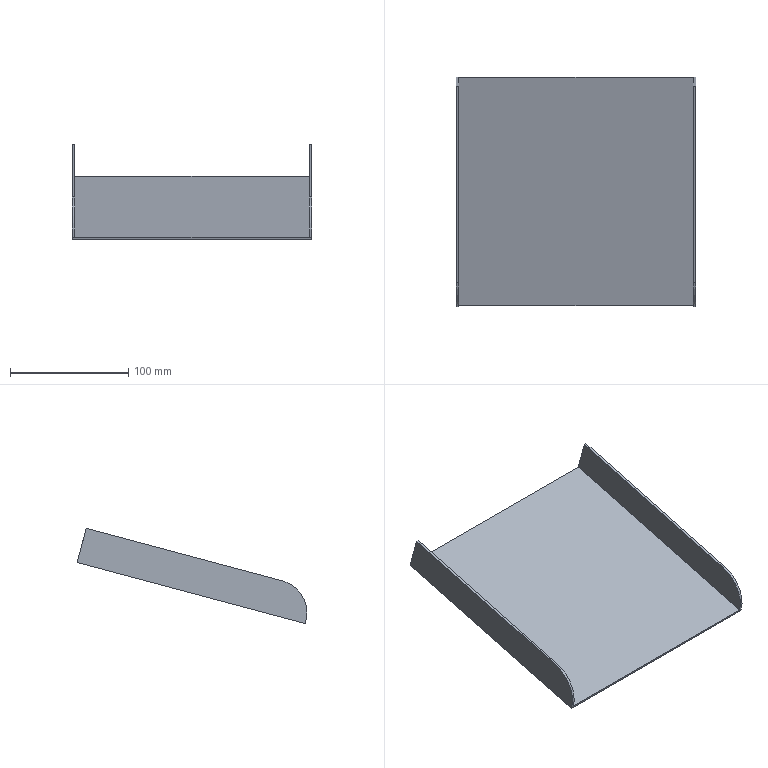Part | NX | features solid 2 | 1 solid | 12 faces | box 203.01 x 194.657 x 80.742 mm | volume 102931 mm3 | plane 10 | cylinder 2 | commonest cylinder face diameters 56 x2
STEP:
#1=CARTESIAN_POINT('',(1038.99,-1003.185,-349.346));
#2=VERTEX_POINT('',#1);
#3=CARTESIAN_POINT('',(1238.,-1003.185,-349.346));
#4=VERTEX_POINT('',#3);
#5=CARTESIAN_POINT('',(1048.99,-1003.185,-349.346));
#6=DIRECTION('',(-1.,0.,0.));
#7=VECTOR('',#6,1000.);
#8=LINE('',#5,#7);
#9=EDGE_CURVE('',#2,#4,#8,.F.);
#10=ORIENTED_EDGE('',*,*,#9,.T.);
#11=CARTESIAN_POINT('',(1238.,-810.,-297.582));
#12=VERTEX_POINT('',#11);
#13=CARTESIAN_POINT('',(1238.,-838.978,-305.347));
#14=DIRECTION('',(0.,0.9659,0.2588));
#15=VECTOR('',#14,1000.);
#16=LINE('',#13,#15);
#17=EDGE_CURVE('',#4,#12,#16,.T.);
#18=ORIENTED_EDGE('',*,*,#17,.T.);
#19=CARTESIAN_POINT('',(1038.99,-810.,-297.582));
#20=VERTEX_POINT('',#19);
#21=CARTESIAN_POINT('',(1048.99,-810.,-297.582));
#22=DIRECTION('',(1.,0.,0.));
#23=VECTOR('',#22,1000.);
#24=LINE('',#21,#23);
#25=EDGE_CURVE('',#20,#12,#24,.T.);
#26=ORIENTED_EDGE('',*,*,#25,.F.);
#27=CARTESIAN_POINT('',(1038.99,-838.978,-305.347));
#28=DIRECTION('',(0.,0.9659,0.2588));
#29=VECTOR('',#28,1000.);
#30=LINE('',#27,#29);
#31=EDGE_CURVE('',#2,#20,#30,.T.);
#32=ORIENTED_EDGE('',*,*,#31,.F.);
#33=EDGE_LOOP('',(#10,#18,#26,#32));
#34=FACE_BOUND('',#33,.T.);
#35=CARTESIAN_POINT('',(1048.99,-838.978,-305.347));
#36=DIRECTION('',(0.,0.2588,-0.9659));
#37=DIRECTION('',(-1.,0.,0.));
#38=AXIS2_PLACEMENT_3D('',#35,#36,#37);
#39=PLANE('',#38);
#40=ADVANCED_FACE('',(#34),#39,.F.);
#41=ORIENTED_EDGE('',*,*,#25,.T.);
#42=CARTESIAN_POINT('',(1238.,-817.247,-270.536));
#43=VERTEX_POINT('',#42);
#44=CARTESIAN_POINT('',(1238.,-809.482,-299.514));
#45=DIRECTION('',(0.,-0.2588,0.9659));
#46=VECTOR('',#45,1000.);
#47=LINE('',#44,#46);
#48=EDGE_CURVE('',#12,#43,#47,.T.);
#49=ORIENTED_EDGE('',*,*,#48,.T.);
#50=CARTESIAN_POINT('',(1240.,-817.247,-270.536));
#51=VERTEX_POINT('',#50);
#52=CARTESIAN_POINT('',(1240.,-817.247,-270.536));
#53=DIRECTION('',(1.,0.,0.));
#54=VECTOR('',#53,1000.);
#55=LINE('',#52,#54);
#56=EDGE_CURVE('',#51,#43,#55,.F.);
#57=ORIENTED_EDGE('',*,*,#56,.F.);
#58=CARTESIAN_POINT('',(1240.,-809.482,-299.514));
#59=VERTEX_POINT('',#58);
#60=CARTESIAN_POINT('',(1240.,-809.482,-299.514));
#61=DIRECTION('',(0.,-0.2588,0.9659));
#62=VECTOR('',#61,1000.);
#63=LINE('',#60,#62);
#64=EDGE_CURVE('',#59,#51,#63,.T.);
#65=ORIENTED_EDGE('',*,*,#64,.F.);
#66=CARTESIAN_POINT('',(1036.99,-809.482,-299.514));
#67=VERTEX_POINT('',#66);
#68=CARTESIAN_POINT('',(1048.99,-809.482,-299.514));
#69=DIRECTION('',(1.,0.,0.));
#70=VECTOR('',#69,1000.);
#71=LINE('',#68,#70);
#72=EDGE_CURVE('',#67,#59,#71,.T.);
#73=ORIENTED_EDGE('',*,*,#72,.F.);
#74=CARTESIAN_POINT('',(1036.99,-817.247,-270.536));
#75=VERTEX_POINT('',#74);
#76=CARTESIAN_POINT('',(1036.99,-809.482,-299.514));
#77=DIRECTION('',(0.,0.2588,-0.9659));
#78=VECTOR('',#77,1000.);
#79=LINE('',#76,#78);
#80=EDGE_CURVE('',#67,#75,#79,.F.);
#81=ORIENTED_EDGE('',*,*,#80,.T.);
#82=CARTESIAN_POINT('',(1038.99,-817.247,-270.536));
#83=VERTEX_POINT('',#82);
#84=CARTESIAN_POINT('',(1036.99,-817.247,-270.536));
#85=DIRECTION('',(1.,0.,0.));
#86=VECTOR('',#85,1000.);
#87=LINE('',#84,#86);
#88=EDGE_CURVE('',#75,#83,#87,.T.);
#89=ORIENTED_EDGE('',*,*,#88,.T.);
#90=CARTESIAN_POINT('',(1038.99,-809.482,-299.514));
#91=DIRECTION('',(0.,-0.2588,0.9659));
#92=VECTOR('',#91,1000.);
#93=LINE('',#90,#92);
#94=EDGE_CURVE('',#20,#83,#93,.T.);
#95=ORIENTED_EDGE('',*,*,#94,.F.);
#96=EDGE_LOOP('',(#41,#49,#57,#65,#73,#81,#89,#95));
#97=FACE_BOUND('',#96,.T.);
#98=CARTESIAN_POINT('',(1048.99,-809.482,-299.514));
#99=DIRECTION('',(0.,0.9659,0.2588));
#100=DIRECTION('',(1.,0.,0.));
#101=AXIS2_PLACEMENT_3D('',#98,#99,#100);
#102=PLANE('',#101);
#103=ADVANCED_FACE('',(#97),#102,.T.);
#104=ORIENTED_EDGE('',*,*,#80,.F.);
#105=CARTESIAN_POINT('',(1036.99,-1002.668,-351.278));
#106=VERTEX_POINT('',#105);
#107=CARTESIAN_POINT('',(1036.99,-838.46,-307.279));
#108=DIRECTION('',(0.,0.9659,0.2588));
#109=VECTOR('',#108,1000.);
#110=LINE('',#107,#109);
#111=EDGE_CURVE('',#67,#106,#110,.F.);
#112=ORIENTED_EDGE('',*,*,#111,.T.);
#113=CARTESIAN_POINT('',(1036.99,-1003.185,-349.346));
#114=VERTEX_POINT('',#113);
#115=CARTESIAN_POINT('',(1036.99,-1002.668,-351.278));
#116=DIRECTION('',(0.,-0.2588,0.9659));
#117=VECTOR('',#116,1000.);
#118=LINE('',#115,#117);
#119=EDGE_CURVE('',#106,#114,#118,.T.);
#120=ORIENTED_EDGE('',*,*,#119,.T.);
#121=CARTESIAN_POINT('',(1036.99,-983.386,-315.053));
#122=VERTEX_POINT('',#121);
#123=CARTESIAN_POINT('',(1036.99,-976.139,-342.099));
#124=DIRECTION('',(-1.,0.,0.));
#125=DIRECTION('',(0.,0.,1.));
#126=AXIS2_PLACEMENT_3D('',#123,#124,#125);
#127=CIRCLE('',#126,28.);
#128=EDGE_CURVE('',#114,#122,#127,.T.);
#129=ORIENTED_EDGE('',*,*,#128,.T.);
#130=CARTESIAN_POINT('',(1036.99,-817.247,-270.536));
#131=DIRECTION('',(0.,-0.9659,-0.2588));
#132=VECTOR('',#131,1000.);
#133=LINE('',#130,#132);
#134=EDGE_CURVE('',#75,#122,#133,.T.);
#135=ORIENTED_EDGE('',*,*,#134,.F.);
#136=EDGE_LOOP('',(#104,#112,#120,#129,#135));
#137=FACE_BOUND('',#136,.T.);
#138=CARTESIAN_POINT('',(1036.99,-838.46,-307.279));
#139=DIRECTION('',(1.,0.,0.));
#140=DIRECTION('',(0.,-0.9659,-0.2588));
#141=AXIS2_PLACEMENT_3D('',#138,#139,#140);
#142=PLANE('',#141);
#143=ADVANCED_FACE('',(#137),#142,.F.);
#144=CARTESIAN_POINT('',(1240.,-1002.668,-351.278));
#145=VERTEX_POINT('',#144);
#146=CARTESIAN_POINT('',(1048.99,-1002.668,-351.278));
#147=DIRECTION('',(1.,0.,0.));
#148=VECTOR('',#147,1000.);
#149=LINE('',#146,#148);
#150=EDGE_CURVE('',#106,#145,#149,.T.);
#151=ORIENTED_EDGE('',*,*,#150,.T.);
#152=CARTESIAN_POINT('',(1240.,-1003.185,-349.346));
#153=VERTEX_POINT('',#152);
#154=CARTESIAN_POINT('',(1240.,-1002.668,-351.278));
#155=DIRECTION('',(0.,0.2588,-0.9659));
#156=VECTOR('',#155,1000.);
#157=LINE('',#154,#156);
#158=EDGE_CURVE('',#145,#153,#157,.F.);
#159=ORIENTED_EDGE('',*,*,#158,.T.);
#160=CARTESIAN_POINT('',(1240.,-1003.185,-349.346));
#161=DIRECTION('',(-1.,0.,0.));
#162=VECTOR('',#161,1000.);
#163=LINE('',#160,#162);
#164=EDGE_CURVE('',#153,#4,#163,.T.);
#165=ORIENTED_EDGE('',*,*,#164,.T.);
#166=ORIENTED_EDGE('',*,*,#9,.F.);
#167=CARTESIAN_POINT('',(1048.99,-1003.185,-349.346));
#168=DIRECTION('',(-1.,0.,0.));
#169=VECTOR('',#168,1000.);
#170=LINE('',#167,#169);
#171=EDGE_CURVE('',#114,#2,#170,.F.);
#172=ORIENTED_EDGE('',*,*,#171,.F.);
#173=ORIENTED_EDGE('',*,*,#119,.F.);
#174=EDGE_LOOP('',(#151,#159,#165,#166,#172,#173));
#175=FACE_BOUND('',#174,.T.);
#176=CARTESIAN_POINT('',(1048.99,-1002.668,-351.278));
#177=DIRECTION('',(0.,0.9659,0.2588));
#178=DIRECTION('',(1.,0.,0.));
#179=AXIS2_PLACEMENT_3D('',#176,#177,#178);
#180=PLANE('',#179);
#181=ADVANCED_FACE('',(#175),#180,.F.);
#182=CARTESIAN_POINT('',(1240.,-838.46,-307.279));
#183=DIRECTION('',(0.,-0.9659,-0.2588));
#184=VECTOR('',#183,1000.);
#185=LINE('',#182,#184);
#186=EDGE_CURVE('',#59,#145,#185,.T.);
#187=ORIENTED_EDGE('',*,*,#186,.F.);
#188=ORIENTED_EDGE('',*,*,#64,.T.);
#189=CARTESIAN_POINT('',(1240.,-983.386,-315.053));
#190=VERTEX_POINT('',#189);
#191=CARTESIAN_POINT('',(1240.,-817.247,-270.536));
#192=DIRECTION('',(0.,-0.9659,-0.2588));
#193=VECTOR('',#192,1000.);
#194=LINE('',#191,#193);
#195=EDGE_CURVE('',#51,#190,#194,.T.);
#196=ORIENTED_EDGE('',*,*,#195,.T.);
#197=CARTESIAN_POINT('',(1240.,-976.139,-342.099));
#198=DIRECTION('',(-1.,0.,0.));
#199=DIRECTION('',(0.,0.,1.));
#200=AXIS2_PLACEMENT_3D('',#197,#198,#199);
#201=CIRCLE('',#200,28.);
#202=EDGE_CURVE('',#190,#153,#201,.F.);
#203=ORIENTED_EDGE('',*,*,#202,.T.);
#204=ORIENTED_EDGE('',*,*,#158,.F.);
#205=EDGE_LOOP('',(#187,#188,#196,#203,#204));
#206=FACE_BOUND('',#205,.T.);
#207=CARTESIAN_POINT('',(1240.,-838.46,-307.279));
#208=DIRECTION('',(1.,0.,0.));
#209=DIRECTION('',(0.,-0.9659,-0.2588));
#210=AXIS2_PLACEMENT_3D('',#207,#208,#209);
#211=PLANE('',#210);
#212=ADVANCED_FACE('',(#206),#211,.T.);
#213=ORIENTED_EDGE('',*,*,#72,.T.);
#214=ORIENTED_EDGE('',*,*,#186,.T.);
#215=ORIENTED_EDGE('',*,*,#150,.F.);
#216=ORIENTED_EDGE('',*,*,#111,.F.);
#217=EDGE_LOOP('',(#213,#214,#215,#216));
#218=FACE_BOUND('',#217,.T.);
#219=CARTESIAN_POINT('',(1048.99,-838.46,-307.279));
#220=DIRECTION('',(0.,0.2588,-0.9659));
#221=DIRECTION('',(-1.,0.,0.));
#222=AXIS2_PLACEMENT_3D('',#219,#220,#221);
#223=PLANE('',#222);
#224=ADVANCED_FACE('',(#218),#223,.T.);
#225=CARTESIAN_POINT('',(1038.99,-983.386,-315.053));
#226=VERTEX_POINT('',#225);
#227=CARTESIAN_POINT('',(1038.99,-976.139,-342.099));
#228=DIRECTION('',(-1.,0.,0.));
#229=DIRECTION('',(0.,0.,1.));
#230=AXIS2_PLACEMENT_3D('',#227,#228,#229);
#231=CIRCLE('',#230,28.);
#232=EDGE_CURVE('',#226,#2,#231,.F.);
#233=ORIENTED_EDGE('',*,*,#232,.T.);
#234=ORIENTED_EDGE('',*,*,#31,.T.);
#235=ORIENTED_EDGE('',*,*,#94,.T.);
#236=CARTESIAN_POINT('',(1038.99,-817.247,-270.536));
#237=DIRECTION('',(0.,-0.9659,-0.2588));
#238=VECTOR('',#237,1000.);
#239=LINE('',#236,#238);
#240=EDGE_CURVE('',#83,#226,#239,.T.);
#241=ORIENTED_EDGE('',*,*,#240,.T.);
#242=EDGE_LOOP('',(#233,#234,#235,#241));
#243=FACE_BOUND('',#242,.T.);
#244=CARTESIAN_POINT('',(1038.99,-809.482,-299.514));
#245=DIRECTION('',(-1.,0.,0.));
#246=DIRECTION('',(0.,0.,1.));
#247=AXIS2_PLACEMENT_3D('',#244,#245,#246);
#248=PLANE('',#247);
#249=ADVANCED_FACE('',(#243),#248,.F.);
#250=ORIENTED_EDGE('',*,*,#134,.T.);
#251=CARTESIAN_POINT('',(1036.99,-983.386,-315.053));
#252=DIRECTION('',(1.,0.,0.));
#253=VECTOR('',#252,1000.);
#254=LINE('',#251,#253);
#255=EDGE_CURVE('',#122,#226,#254,.T.);
#256=ORIENTED_EDGE('',*,*,#255,.T.);
#257=ORIENTED_EDGE('',*,*,#240,.F.);
#258=ORIENTED_EDGE('',*,*,#88,.F.);
#259=EDGE_LOOP('',(#250,#256,#257,#258));
#260=FACE_BOUND('',#259,.T.);
#261=CARTESIAN_POINT('',(1036.99,-817.247,-270.536));
#262=DIRECTION('',(0.,0.2588,-0.9659));
#263=DIRECTION('',(0.,-0.9659,-0.2588));
#264=AXIS2_PLACEMENT_3D('',#261,#262,#263);
#265=PLANE('',#264);
#266=ADVANCED_FACE('',(#260),#265,.F.);
#267=ORIENTED_EDGE('',*,*,#128,.F.);
#268=ORIENTED_EDGE('',*,*,#171,.T.);
#269=ORIENTED_EDGE('',*,*,#232,.F.);
#270=ORIENTED_EDGE('',*,*,#255,.F.);
#271=EDGE_LOOP('',(#267,#268,#269,#270));
#272=FACE_BOUND('',#271,.T.);
#273=CARTESIAN_POINT('',(1036.99,-976.139,-342.099));
#274=DIRECTION('',(-1.,0.,0.));
#275=DIRECTION('',(0.,0.,1.));
#276=AXIS2_PLACEMENT_3D('',#273,#274,#275);
#277=CYLINDRICAL_SURFACE('',#276,28.);
#278=ADVANCED_FACE('',(#272),#277,.T.);
#279=ORIENTED_EDGE('',*,*,#17,.F.);
#280=CARTESIAN_POINT('',(1238.,-983.386,-315.053));
#281=VERTEX_POINT('',#280);
#282=CARTESIAN_POINT('',(1238.,-976.139,-342.099));
#283=DIRECTION('',(-1.,0.,0.));
#284=DIRECTION('',(0.,0.,1.));
#285=AXIS2_PLACEMENT_3D('',#282,#283,#284);
#286=CIRCLE('',#285,28.);
#287=EDGE_CURVE('',#4,#281,#286,.T.);
#288=ORIENTED_EDGE('',*,*,#287,.T.);
#289=CARTESIAN_POINT('',(1238.,-817.247,-270.536));
#290=DIRECTION('',(0.,-0.9659,-0.2588));
#291=VECTOR('',#290,1000.);
#292=LINE('',#289,#291);
#293=EDGE_CURVE('',#43,#281,#292,.T.);
#294=ORIENTED_EDGE('',*,*,#293,.F.);
#295=ORIENTED_EDGE('',*,*,#48,.F.);
#296=EDGE_LOOP('',(#279,#288,#294,#295));
#297=FACE_BOUND('',#296,.T.);
#298=CARTESIAN_POINT('',(1238.,-809.482,-299.514));
#299=DIRECTION('',(-1.,0.,0.));
#300=DIRECTION('',(0.,0.,1.));
#301=AXIS2_PLACEMENT_3D('',#298,#299,#300);
#302=PLANE('',#301);
#303=ADVANCED_FACE('',(#297),#302,.T.);
#304=ORIENTED_EDGE('',*,*,#293,.T.);
#305=CARTESIAN_POINT('',(1240.,-983.386,-315.053));
#306=DIRECTION('',(1.,0.,0.));
#307=VECTOR('',#306,1000.);
#308=LINE('',#305,#307);
#309=EDGE_CURVE('',#281,#190,#308,.T.);
#310=ORIENTED_EDGE('',*,*,#309,.T.);
#311=ORIENTED_EDGE('',*,*,#195,.F.);
#312=ORIENTED_EDGE('',*,*,#56,.T.);
#313=EDGE_LOOP('',(#304,#310,#311,#312));
#314=FACE_BOUND('',#313,.T.);
#315=CARTESIAN_POINT('',(1240.,-817.247,-270.536));
#316=DIRECTION('',(0.,0.2588,-0.9659));
#317=DIRECTION('',(0.,-0.9659,-0.2588));
#318=AXIS2_PLACEMENT_3D('',#315,#316,#317);
#319=PLANE('',#318);
#320=ADVANCED_FACE('',(#314),#319,.F.);
#321=ORIENTED_EDGE('',*,*,#202,.F.);
#322=ORIENTED_EDGE('',*,*,#309,.F.);
#323=ORIENTED_EDGE('',*,*,#287,.F.);
#324=ORIENTED_EDGE('',*,*,#164,.F.);
#325=EDGE_LOOP('',(#321,#322,#323,#324));
#326=FACE_BOUND('',#325,.T.);
#327=CARTESIAN_POINT('',(1240.,-976.139,-342.099));
#328=DIRECTION('',(1.,0.,0.));
#329=DIRECTION('',(0.,0.,-1.));
#330=AXIS2_PLACEMENT_3D('',#327,#328,#329);
#331=CYLINDRICAL_SURFACE('',#330,28.);
#332=ADVANCED_FACE('',(#326),#331,.T.);
#333=CLOSED_SHELL('',(#40,#103,#143,#181,#212,#224,#249,#266,#278,#303,#320,#332));
#334=MANIFOLD_SOLID_BREP('',#333);
#335=(LENGTH_UNIT()NAMED_UNIT(*)SI_UNIT(.MILLI.,.METRE.));
#336=UNCERTAINTY_MEASURE_WITH_UNIT(LENGTH_MEASURE(0.00001),#335,'','');
#337=(NAMED_UNIT(*)PLANE_ANGLE_UNIT()SI_UNIT($,.RADIAN.));
#338=(NAMED_UNIT(*)SI_UNIT($,.STERADIAN.)SOLID_ANGLE_UNIT());
#339=(GEOMETRIC_REPRESENTATION_CONTEXT(3)GLOBAL_UNCERTAINTY_ASSIGNED_CONTEXT((#336))GLOBAL_UNIT_ASSIGNED_CONTEXT((#335,#337,#338))REPRESENTATION_CONTEXT('',''));
#340=ADVANCED_BREP_SHAPE_REPRESENTATION('',(#334),#339);